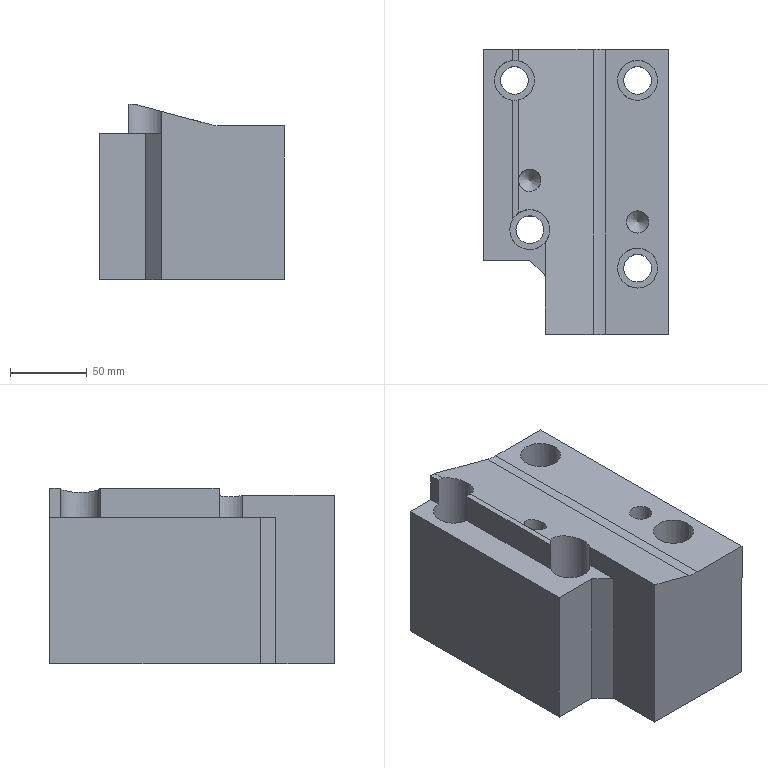Part | STEP file | lll_id5062_x_t | 1 solid | 41 faces | box 120 x 185 x 114 mm | volume 1880331 mm3 | plane 22 | cylinder 15 | cone 2 | torus 2 | commonest cylinder face diameters 18.009 x4 26.008 x4 2 x2 14.506 x2 25 x2 60 x1
STEP:
#1=CARTESIAN_POINT('',(1663.,76.687,-5.));
#2=VERTEX_POINT('',#1);
#3=CARTESIAN_POINT('',(1663.,55.,-5.));
#4=VERTEX_POINT('',#3);
#5=CARTESIAN_POINT('',(1663.,111.,-5.));
#6=DIRECTION('',(0.,-1.,0.));
#7=VECTOR('',#6,1.);
#8=LINE('',#5,#7);
#9=EDGE_CURVE('',#2,#4,#8,.T.);
#10=ORIENTED_EDGE('',*,*,#9,.T.);
#11=CARTESIAN_POINT('',(1663.,55.,-100.));
#12=VERTEX_POINT('',#11);
#13=CARTESIAN_POINT('',(1663.,55.,-80.));
#14=DIRECTION('',(0.,0.,-1.));
#15=VECTOR('',#14,1.);
#16=LINE('',#13,#15);
#17=EDGE_CURVE('',#4,#12,#16,.T.);
#18=ORIENTED_EDGE('',*,*,#17,.T.);
#19=CARTESIAN_POINT('',(1663.,17.,-100.));
#20=VERTEX_POINT('',#19);
#21=CARTESIAN_POINT('',(1663.,111.,-100.));
#22=DIRECTION('',(0.,-1.,0.));
#23=VECTOR('',#22,1.);
#24=LINE('',#21,#23);
#25=EDGE_CURVE('',#12,#20,#24,.T.);
#26=ORIENTED_EDGE('',*,*,#25,.T.);
#27=CARTESIAN_POINT('',(1663.,17.,9.362));
#28=VERTEX_POINT('',#27);
#29=CARTESIAN_POINT('',(1663.,17.,-42.5));
#30=DIRECTION('',(0.,0.,1.));
#31=VECTOR('',#30,1.);
#32=LINE('',#29,#31);
#33=EDGE_CURVE('',#20,#28,#32,.T.);
#34=ORIENTED_EDGE('',*,*,#33,.T.);
#35=CARTESIAN_POINT('',(1663.,76.687,9.362));
#36=VERTEX_POINT('',#35);
#37=CARTESIAN_POINT('',(1663.,22.5,9.362));
#38=DIRECTION('',(0.,1.,0.));
#39=VECTOR('',#38,1.);
#40=LINE('',#37,#39);
#41=EDGE_CURVE('',#28,#36,#40,.T.);
#42=ORIENTED_EDGE('',*,*,#41,.T.);
#43=CARTESIAN_POINT('',(1663.,76.687,3.53));
#44=DIRECTION('',(0.,0.,1.));
#45=VECTOR('',#44,1.);
#46=LINE('',#43,#45);
#47=EDGE_CURVE('',#2,#36,#46,.T.);
#48=ORIENTED_EDGE('',*,*,#47,.F.);
#49=EDGE_LOOP('',(#10,#18,#26,#34,#42,#48));
#50=FACE_OUTER_BOUND('',#49,.T.);
#51=CARTESIAN_POINT('',(1663.,111.,-42.5));
#52=DIRECTION('',(-1.,0.,0.));
#53=DIRECTION('',(0.,0.,-1.));
#54=AXIS2_PLACEMENT_3D('',#51,#52,#53);
#55=PLANE('',#54);
#56=ADVANCED_FACE('',(#50),#55,.T.);
#57=CARTESIAN_POINT('',(1645.691,202.,14.));
#58=VERTEX_POINT('',#57);
#59=CARTESIAN_POINT('',(1642.,202.,14.));
#60=VERTEX_POINT('',#59);
#61=CARTESIAN_POINT('',(1674.,202.,14.));
#62=DIRECTION('',(-1.,0.,0.));
#63=VECTOR('',#62,1.);
#64=LINE('',#61,#63);
#65=EDGE_CURVE('',#58,#60,#64,.T.);
#66=ORIENTED_EDGE('',*,*,#65,.F.);
#67=CARTESIAN_POINT('',(1694.125,202.,1.022));
#68=VERTEX_POINT('',#67);
#69=CARTESIAN_POINT('',(1773.773,202.,-20.319));
#70=DIRECTION('',(0.9659,0.,-0.2588));
#71=VECTOR('',#70,1.);
#72=LINE('',#69,#71);
#73=EDGE_CURVE('',#58,#68,#72,.T.);
#74=ORIENTED_EDGE('',*,*,#73,.T.);
#75=CARTESIAN_POINT('',(1701.89,202.,0.));
#76=VERTEX_POINT('',#75);
#77=CARTESIAN_POINT('',(1701.89,202.,30.));
#78=DIRECTION('',(0.,1.,0.));
#79=DIRECTION('',(0.,0.,1.));
#80=AXIS2_PLACEMENT_3D('',#77,#78,#79);
#81=CIRCLE('',#80,30.);
#82=EDGE_CURVE('',#76,#68,#81,.T.);
#83=ORIENTED_EDGE('',*,*,#82,.F.);
#84=CARTESIAN_POINT('',(1743.,202.,0.));
#85=VERTEX_POINT('',#84);
#86=CARTESIAN_POINT('',(12283.883,202.,0.));
#87=DIRECTION('',(1.,0.,0.));
#88=VECTOR('',#87,1.);
#89=LINE('',#86,#88);
#90=EDGE_CURVE('',#76,#85,#89,.T.);
#91=ORIENTED_EDGE('',*,*,#90,.T.);
#92=CARTESIAN_POINT('',(1743.,202.,-100.));
#93=VERTEX_POINT('',#92);
#94=CARTESIAN_POINT('',(1743.,202.,-32.057));
#95=DIRECTION('',(0.,0.,-1.));
#96=VECTOR('',#95,1.);
#97=LINE('',#94,#96);
#98=EDGE_CURVE('',#85,#93,#97,.T.);
#99=ORIENTED_EDGE('',*,*,#98,.T.);
#100=CARTESIAN_POINT('',(1623.,202.,-100.));
#101=VERTEX_POINT('',#100);
#102=CARTESIAN_POINT('',(1674.,202.,-100.));
#103=DIRECTION('',(-1.,0.,0.));
#104=VECTOR('',#103,1.);
#105=LINE('',#102,#104);
#106=EDGE_CURVE('',#93,#101,#105,.T.);
#107=ORIENTED_EDGE('',*,*,#106,.T.);
#108=CARTESIAN_POINT('',(1623.,202.,-5.));
#109=VERTEX_POINT('',#108);
#110=CARTESIAN_POINT('',(1623.,202.,-80.));
#111=DIRECTION('',(0.,0.,-1.));
#112=VECTOR('',#111,1.);
#113=LINE('',#110,#112);
#114=EDGE_CURVE('',#109,#101,#113,.T.);
#115=ORIENTED_EDGE('',*,*,#114,.F.);
#116=CARTESIAN_POINT('',(1642.,202.,-5.));
#117=VERTEX_POINT('',#116);
#118=CARTESIAN_POINT('',(1674.,202.,-5.));
#119=DIRECTION('',(1.,0.,0.));
#120=VECTOR('',#119,1.);
#121=LINE('',#118,#120);
#122=EDGE_CURVE('',#109,#117,#121,.T.);
#123=ORIENTED_EDGE('',*,*,#122,.T.);
#124=CARTESIAN_POINT('',(1642.,202.,-33.25));
#125=DIRECTION('',(0.,0.,-1.));
#126=VECTOR('',#125,1.);
#127=LINE('',#124,#126);
#128=EDGE_CURVE('',#60,#117,#127,.T.);
#129=ORIENTED_EDGE('',*,*,#128,.F.);
#130=EDGE_LOOP('',(#66,#74,#83,#91,#99,#107,#115,#123,#129));
#131=FACE_OUTER_BOUND('',#130,.T.);
#132=CARTESIAN_POINT('',(1674.,202.,-34.988));
#133=DIRECTION('',(0.,1.,0.));
#134=DIRECTION('',(0.,0.,-1.));
#135=AXIS2_PLACEMENT_3D('',#132,#133,#134);
#136=PLANE('',#135);
#137=ADVANCED_FACE('',(#131),#136,.T.);
#138=CARTESIAN_POINT('',(1694.125,17.,1.022));
#139=VERTEX_POINT('',#138);
#140=CARTESIAN_POINT('',(1773.773,17.,-20.319));
#141=DIRECTION('',(-0.9659,0.,0.2588));
#142=VECTOR('',#141,1.);
#143=LINE('',#140,#142);
#144=EDGE_CURVE('',#139,#28,#143,.T.);
#145=ORIENTED_EDGE('',*,*,#144,.T.);
#146=ORIENTED_EDGE('',*,*,#33,.F.);
#147=CARTESIAN_POINT('',(1743.,17.,-100.));
#148=VERTEX_POINT('',#147);
#149=CARTESIAN_POINT('',(1644.,17.,-100.));
#150=DIRECTION('',(1.,0.,0.));
#151=VECTOR('',#150,1.);
#152=LINE('',#149,#151);
#153=EDGE_CURVE('',#20,#148,#152,.T.);
#154=ORIENTED_EDGE('',*,*,#153,.T.);
#155=CARTESIAN_POINT('',(1743.,17.,0.));
#156=VERTEX_POINT('',#155);
#157=CARTESIAN_POINT('',(1743.,17.,-80.));
#158=DIRECTION('',(0.,0.,-1.));
#159=VECTOR('',#158,1.);
#160=LINE('',#157,#159);
#161=EDGE_CURVE('',#156,#148,#160,.T.);
#162=ORIENTED_EDGE('',*,*,#161,.F.);
#163=CARTESIAN_POINT('',(1701.89,17.,0.));
#164=VERTEX_POINT('',#163);
#165=CARTESIAN_POINT('',(12283.883,17.,0.));
#166=DIRECTION('',(-1.,0.,0.));
#167=VECTOR('',#166,1.);
#168=LINE('',#165,#167);
#169=EDGE_CURVE('',#156,#164,#168,.T.);
#170=ORIENTED_EDGE('',*,*,#169,.T.);
#171=CARTESIAN_POINT('',(1701.89,17.,30.));
#172=DIRECTION('',(0.,1.,0.));
#173=DIRECTION('',(0.,0.,-1.));
#174=AXIS2_PLACEMENT_3D('',#171,#172,#173);
#175=CIRCLE('',#174,30.);
#176=EDGE_CURVE('',#164,#139,#175,.T.);
#177=ORIENTED_EDGE('',*,*,#176,.T.);
#178=EDGE_LOOP('',(#145,#146,#154,#162,#170,#177));
#179=FACE_OUTER_BOUND('',#178,.T.);
#180=CARTESIAN_POINT('',(1644.,17.,-80.));
#181=DIRECTION('',(0.,-1.,0.));
#182=DIRECTION('',(0.,0.,1.));
#183=AXIS2_PLACEMENT_3D('',#180,#181,#182);
#184=PLANE('',#183);
#185=ADVANCED_FACE('',(#179),#184,.T.);
#186=ORIENTED_EDGE('',*,*,#73,.F.);
#187=CARTESIAN_POINT('',(1645.691,194.722,14.));
#188=VERTEX_POINT('',#187);
#189=CARTESIAN_POINT('',(1645.691,22.5,14.));
#190=DIRECTION('',(0.,-1.,0.));
#191=VECTOR('',#190,1.);
#192=LINE('',#189,#191);
#193=EDGE_CURVE('',#58,#188,#192,.T.);
#194=ORIENTED_EDGE('',*,*,#193,.T.);
#195=CARTESIAN_POINT('',(1645.691,169.277,14.));
#196=VERTEX_POINT('',#195);
#197=CARTESIAN_POINT('',(1643.,182.,14.721));
#198=DIRECTION('',(-0.2588,0.,-0.9659));
#199=DIRECTION('',(0.9659,0.,-0.2588));
#200=AXIS2_PLACEMENT_3D('',#197,#198,#199);
#201=ELLIPSE('',#200,13.463,13.004);
#202=EDGE_CURVE('',#188,#196,#201,.T.);
#203=ORIENTED_EDGE('',*,*,#202,.T.);
#204=CARTESIAN_POINT('',(1645.691,95.756,14.));
#205=VERTEX_POINT('',#204);
#206=CARTESIAN_POINT('',(1645.691,22.5,14.));
#207=DIRECTION('',(0.,-1.,0.));
#208=VECTOR('',#207,1.);
#209=LINE('',#206,#208);
#210=EDGE_CURVE('',#196,#205,#209,.T.);
#211=ORIENTED_EDGE('',*,*,#210,.T.);
#212=CARTESIAN_POINT('',(1653.,85.,12.042));
#213=DIRECTION('',(-0.2588,0.,-0.9659));
#214=DIRECTION('',(0.9659,0.,-0.2588));
#215=AXIS2_PLACEMENT_3D('',#212,#213,#214);
#216=ELLIPSE('',#215,13.463,13.004);
#217=EDGE_CURVE('',#205,#36,#216,.T.);
#218=ORIENTED_EDGE('',*,*,#217,.T.);
#219=ORIENTED_EDGE('',*,*,#41,.F.);
#220=ORIENTED_EDGE('',*,*,#144,.F.);
#221=CARTESIAN_POINT('',(1694.125,22.5,1.022));
#222=DIRECTION('',(0.,-1.,0.));
#223=VECTOR('',#222,1.);
#224=LINE('',#221,#223);
#225=EDGE_CURVE('',#68,#139,#224,.T.);
#226=ORIENTED_EDGE('',*,*,#225,.F.);
#227=EDGE_LOOP('',(#186,#194,#203,#211,#218,#219,#220,#226));
#228=FACE_BOUND('',#227,.T.);
#229=CARTESIAN_POINT('',(1660.253,117.,10.098));
#230=VERTEX_POINT('',#229);
#231=CARTESIAN_POINT('',(1653.,117.,12.042));
#232=DIRECTION('',(-0.2588,0.,-0.9659));
#233=DIRECTION('',(0.9659,0.,-0.2588));
#234=AXIS2_PLACEMENT_3D('',#231,#232,#233);
#235=ELLIPSE('',#234,7.509,7.253);
#236=EDGE_CURVE('',#230,#230,#235,.T.);
#237=ORIENTED_EDGE('',*,*,#236,.T.);
#238=EDGE_LOOP('',(#237));
#239=FACE_BOUND('',#238,.T.);
#240=CARTESIAN_POINT('',(1773.773,22.5,-20.319));
#241=DIRECTION('',(-0.2588,0.,-0.9659));
#242=DIRECTION('',(0.9659,0.,-0.2588));
#243=AXIS2_PLACEMENT_3D('',#240,#241,#242);
#244=PLANE('',#243);
#245=ADVANCED_FACE('',(#228,#239),#244,.F.);
#246=CARTESIAN_POINT('',(1660.,122.,-100.));
#247=VERTEX_POINT('',#246);
#248=CARTESIAN_POINT('',(1660.,147.,-100.));
#249=VERTEX_POINT('',#248);
#250=CARTESIAN_POINT('',(1660.,134.5,-100.));
#251=DIRECTION('',(0.,0.,-1.));
#252=DIRECTION('',(-1.,0.,0.));
#253=AXIS2_PLACEMENT_3D('',#250,#251,#252);
#254=CIRCLE('',#253,12.5);
#255=EDGE_CURVE('',#247,#249,#254,.T.);
#256=ORIENTED_EDGE('',*,*,#255,.F.);
#257=CARTESIAN_POINT('',(1716.,122.,-100.));
#258=VERTEX_POINT('',#257);
#259=CARTESIAN_POINT('',(-2196.249,122.,-100.));
#260=DIRECTION('',(-1.,0.,0.));
#261=VECTOR('',#260,1.);
#262=LINE('',#259,#261);
#263=EDGE_CURVE('',#258,#247,#262,.T.);
#264=ORIENTED_EDGE('',*,*,#263,.F.);
#265=CARTESIAN_POINT('',(1716.,147.,-100.));
#266=VERTEX_POINT('',#265);
#267=CARTESIAN_POINT('',(1716.,134.5,-100.));
#268=DIRECTION('',(0.,0.,-1.));
#269=DIRECTION('',(-1.,0.,0.));
#270=AXIS2_PLACEMENT_3D('',#267,#268,#269);
#271=CIRCLE('',#270,12.5);
#272=EDGE_CURVE('',#266,#258,#271,.T.);
#273=ORIENTED_EDGE('',*,*,#272,.F.);
#274=CARTESIAN_POINT('',(-2196.249,147.,-100.));
#275=DIRECTION('',(1.,0.,0.));
#276=VECTOR('',#275,1.);
#277=LINE('',#274,#276);
#278=EDGE_CURVE('',#249,#266,#277,.T.);
#279=ORIENTED_EDGE('',*,*,#278,.F.);
#280=EDGE_LOOP('',(#256,#264,#273,#279));
#281=FACE_BOUND('',#280,.T.);
#282=CARTESIAN_POINT('',(1713.995,182.,-100.));
#283=VERTEX_POINT('',#282);
#284=CARTESIAN_POINT('',(1723.,182.,-100.));
#285=DIRECTION('',(0.,0.,-1.));
#286=DIRECTION('',(-1.,0.,0.));
#287=AXIS2_PLACEMENT_3D('',#284,#285,#286);
#288=CIRCLE('',#287,9.005);
#289=EDGE_CURVE('',#283,#283,#288,.T.);
#290=ORIENTED_EDGE('',*,*,#289,.F.);
#291=EDGE_LOOP('',(#290));
#292=FACE_BOUND('',#291,.T.);
#293=CARTESIAN_POINT('',(1713.995,60.,-100.));
#294=VERTEX_POINT('',#293);
#295=CARTESIAN_POINT('',(1723.,60.,-100.));
#296=DIRECTION('',(0.,0.,-1.));
#297=DIRECTION('',(-1.,0.,0.));
#298=AXIS2_PLACEMENT_3D('',#295,#296,#297);
#299=CIRCLE('',#298,9.005);
#300=EDGE_CURVE('',#294,#294,#299,.T.);
#301=ORIENTED_EDGE('',*,*,#300,.F.);
#302=EDGE_LOOP('',(#301));
#303=FACE_BOUND('',#302,.T.);
#304=ORIENTED_EDGE('',*,*,#153,.F.);
#305=ORIENTED_EDGE('',*,*,#25,.F.);
#306=CARTESIAN_POINT('',(1653.,65.,-100.));
#307=VERTEX_POINT('',#306);
#308=CARTESIAN_POINT('',(1653.,65.,-100.));
#309=DIRECTION('',(-0.7071,0.7071,0.));
#310=VECTOR('',#309,1.);
#311=LINE('',#308,#310);
#312=EDGE_CURVE('',#12,#307,#311,.T.);
#313=ORIENTED_EDGE('',*,*,#312,.T.);
#314=CARTESIAN_POINT('',(1623.,65.,-100.));
#315=VERTEX_POINT('',#314);
#316=CARTESIAN_POINT('',(1644.,65.,-100.));
#317=DIRECTION('',(1.,0.,0.));
#318=VECTOR('',#317,1.);
#319=LINE('',#316,#318);
#320=EDGE_CURVE('',#315,#307,#319,.T.);
#321=ORIENTED_EDGE('',*,*,#320,.F.);
#322=CARTESIAN_POINT('',(1623.,320.,-100.));
#323=DIRECTION('',(0.,-1.,0.));
#324=VECTOR('',#323,1.);
#325=LINE('',#322,#324);
#326=EDGE_CURVE('',#101,#315,#325,.T.);
#327=ORIENTED_EDGE('',*,*,#326,.F.);
#328=ORIENTED_EDGE('',*,*,#106,.F.);
#329=CARTESIAN_POINT('',(1743.,187.,-100.));
#330=DIRECTION('',(0.,-1.,0.));
#331=VECTOR('',#330,1.);
#332=LINE('',#329,#331);
#333=EDGE_CURVE('',#93,#148,#332,.T.);
#334=ORIENTED_EDGE('',*,*,#333,.T.);
#335=EDGE_LOOP('',(#304,#305,#313,#321,#327,#328,#334));
#336=FACE_BOUND('',#335,.T.);
#337=CARTESIAN_POINT('',(1643.995,85.,-100.));
#338=VERTEX_POINT('',#337);
#339=CARTESIAN_POINT('',(1653.,85.,-100.));
#340=DIRECTION('',(0.,0.,-1.));
#341=DIRECTION('',(-1.,0.,0.));
#342=AXIS2_PLACEMENT_3D('',#339,#340,#341);
#343=CIRCLE('',#342,9.005);
#344=EDGE_CURVE('',#338,#338,#343,.T.);
#345=ORIENTED_EDGE('',*,*,#344,.F.);
#346=EDGE_LOOP('',(#345));
#347=FACE_BOUND('',#346,.T.);
#348=CARTESIAN_POINT('',(1633.995,182.,-100.));
#349=VERTEX_POINT('',#348);
#350=CARTESIAN_POINT('',(1643.,182.,-100.));
#351=DIRECTION('',(0.,0.,-1.));
#352=DIRECTION('',(-1.,0.,0.));
#353=AXIS2_PLACEMENT_3D('',#350,#351,#352);
#354=CIRCLE('',#353,9.005);
#355=EDGE_CURVE('',#349,#349,#354,.T.);
#356=ORIENTED_EDGE('',*,*,#355,.F.);
#357=EDGE_LOOP('',(#356));
#358=FACE_BOUND('',#357,.T.);
#359=CARTESIAN_POINT('',(-2196.249,1.,-100.));
#360=DIRECTION('',(0.,0.,-1.));
#361=DIRECTION('',(1.,0.,0.));
#362=AXIS2_PLACEMENT_3D('',#359,#360,#361);
#363=PLANE('',#362);
#364=ADVANCED_FACE('',(#281,#292,#303,#336,#347,#358),#363,.T.);
#365=ORIENTED_EDGE('',*,*,#217,.F.);
#366=CARTESIAN_POINT('',(1642.,91.936,14.));
#367=VERTEX_POINT('',#366);
#368=CARTESIAN_POINT('',(1653.,85.,14.));
#369=DIRECTION('',(0.,0.,-1.));
#370=DIRECTION('',(-1.,0.,0.));
#371=AXIS2_PLACEMENT_3D('',#368,#369,#370);
#372=CIRCLE('',#371,13.004);
#373=EDGE_CURVE('',#367,#205,#372,.T.);
#374=ORIENTED_EDGE('',*,*,#373,.F.);
#375=CARTESIAN_POINT('',(1642.,91.936,-5.));
#376=VERTEX_POINT('',#375);
#377=CARTESIAN_POINT('',(1642.,91.936,13.5));
#378=DIRECTION('',(0.,0.,-1.));
#379=VECTOR('',#378,1.);
#380=LINE('',#377,#379);
#381=EDGE_CURVE('',#367,#376,#380,.T.);
#382=ORIENTED_EDGE('',*,*,#381,.T.);
#383=CARTESIAN_POINT('',(1653.,85.,-5.));
#384=DIRECTION('',(0.,0.,1.));
#385=DIRECTION('',(1.,0.,0.));
#386=AXIS2_PLACEMENT_3D('',#383,#384,#385);
#387=CIRCLE('',#386,13.004);
#388=EDGE_CURVE('',#376,#2,#387,.T.);
#389=ORIENTED_EDGE('',*,*,#388,.T.);
#390=ORIENTED_EDGE('',*,*,#47,.T.);
#391=EDGE_LOOP('',(#365,#374,#382,#389,#390));
#392=FACE_BOUND('',#391,.T.);
#393=CARTESIAN_POINT('',(1639.996,85.,-50.));
#394=VERTEX_POINT('',#393);
#395=CARTESIAN_POINT('',(1653.,85.,-50.));
#396=DIRECTION('',(0.,0.,-1.));
#397=DIRECTION('',(-1.,0.,0.));
#398=AXIS2_PLACEMENT_3D('',#395,#396,#397);
#399=CIRCLE('',#398,13.004);
#400=EDGE_CURVE('',#394,#394,#399,.T.);
#401=ORIENTED_EDGE('',*,*,#400,.T.);
#402=EDGE_LOOP('',(#401));
#403=FACE_BOUND('',#402,.T.);
#404=CARTESIAN_POINT('',(1653.,85.,13.5));
#405=DIRECTION('',(0.,0.,-1.));
#406=DIRECTION('',(-1.,0.,0.));
#407=AXIS2_PLACEMENT_3D('',#404,#405,#406);
#408=CYLINDRICAL_SURFACE('',#407,13.004);
#409=ADVANCED_FACE('',(#392,#403),#408,.F.);
#410=ORIENTED_EDGE('',*,*,#400,.F.);
#411=EDGE_LOOP('',(#410));
#412=FACE_BOUND('',#411,.T.);
#413=CARTESIAN_POINT('',(1662.005,85.,-50.));
#414=VERTEX_POINT('',#413);
#415=CARTESIAN_POINT('',(1653.,85.,-50.));
#416=DIRECTION('',(0.,0.,-1.));
#417=DIRECTION('',(1.,0.,0.));
#418=AXIS2_PLACEMENT_3D('',#415,#416,#417);
#419=CIRCLE('',#418,9.005);
#420=EDGE_CURVE('',#414,#414,#419,.T.);
#421=ORIENTED_EDGE('',*,*,#420,.T.);
#422=EDGE_LOOP('',(#421));
#423=FACE_BOUND('',#422,.T.);
#424=CARTESIAN_POINT('',(1653.,85.,-50.));
#425=DIRECTION('',(0.,0.,-1.));
#426=DIRECTION('',(1.,0.,0.));
#427=AXIS2_PLACEMENT_3D('',#424,#425,#426);
#428=PLANE('',#427);
#429=ADVANCED_FACE('',(#412,#423),#428,.F.);
#430=ORIENTED_EDGE('',*,*,#98,.F.);
#431=CARTESIAN_POINT('',(1743.,-13712.786,0.));
#432=DIRECTION('',(0.,1.,0.));
#433=VECTOR('',#432,1.);
#434=LINE('',#431,#433);
#435=EDGE_CURVE('',#156,#85,#434,.T.);
#436=ORIENTED_EDGE('',*,*,#435,.F.);
#437=ORIENTED_EDGE('',*,*,#161,.T.);
#438=ORIENTED_EDGE('',*,*,#333,.F.);
#439=EDGE_LOOP('',(#430,#436,#437,#438));
#440=FACE_OUTER_BOUND('',#439,.T.);
#441=CARTESIAN_POINT('',(1743.,187.,-32.057));
#442=DIRECTION('',(-1.,0.,0.));
#443=DIRECTION('',(0.,0.,-1.));
#444=AXIS2_PLACEMENT_3D('',#441,#442,#443);
#445=PLANE('',#444);
#446=ADVANCED_FACE('',(#440),#445,.F.);
#447=CARTESIAN_POINT('',(1723.,82.747,0.));
#448=VERTEX_POINT('',#447);
#449=CARTESIAN_POINT('',(1723.,90.,0.));
#450=DIRECTION('',(0.,0.,-1.));
#451=DIRECTION('',(0.,-1.,0.));
#452=AXIS2_PLACEMENT_3D('',#449,#450,#451);
#453=CIRCLE('',#452,7.253);
#454=EDGE_CURVE('',#448,#448,#453,.T.);
#455=ORIENTED_EDGE('',*,*,#454,.T.);
#456=EDGE_LOOP('',(#455));
#457=FACE_BOUND('',#456,.T.);
#458=CARTESIAN_POINT('',(1723.,168.996,0.));
#459=VERTEX_POINT('',#458);
#460=CARTESIAN_POINT('',(1723.,182.,0.));
#461=DIRECTION('',(0.,0.,-1.));
#462=DIRECTION('',(0.,-1.,0.));
#463=AXIS2_PLACEMENT_3D('',#460,#461,#462);
#464=CIRCLE('',#463,13.004);
#465=EDGE_CURVE('',#459,#459,#464,.T.);
#466=ORIENTED_EDGE('',*,*,#465,.T.);
#467=EDGE_LOOP('',(#466));
#468=FACE_BOUND('',#467,.T.);
#469=CARTESIAN_POINT('',(1723.,46.996,0.));
#470=VERTEX_POINT('',#469);
#471=CARTESIAN_POINT('',(1723.,60.,0.));
#472=DIRECTION('',(0.,0.,-1.));
#473=DIRECTION('',(0.,-1.,0.));
#474=AXIS2_PLACEMENT_3D('',#471,#472,#473);
#475=CIRCLE('',#474,13.004);
#476=EDGE_CURVE('',#470,#470,#475,.T.);
#477=ORIENTED_EDGE('',*,*,#476,.T.);
#478=EDGE_LOOP('',(#477));
#479=FACE_BOUND('',#478,.T.);
#480=ORIENTED_EDGE('',*,*,#90,.F.);
#481=CARTESIAN_POINT('',(1701.89,22.5,0.));
#482=DIRECTION('',(0.,-1.,0.));
#483=VECTOR('',#482,1.);
#484=LINE('',#481,#483);
#485=EDGE_CURVE('',#76,#164,#484,.T.);
#486=ORIENTED_EDGE('',*,*,#485,.T.);
#487=ORIENTED_EDGE('',*,*,#169,.F.);
#488=ORIENTED_EDGE('',*,*,#435,.T.);
#489=EDGE_LOOP('',(#480,#486,#487,#488));
#490=FACE_BOUND('',#489,.T.);
#491=CARTESIAN_POINT('',(12283.883,-13712.786,0.));
#492=DIRECTION('',(0.,0.,-1.));
#493=DIRECTION('',(1.,0.,0.));
#494=AXIS2_PLACEMENT_3D('',#491,#492,#493);
#495=PLANE('',#494);
#496=ADVANCED_FACE('',(#457,#468,#479,#490),#495,.F.);
#497=ORIENTED_EDGE('',*,*,#82,.T.);
#498=ORIENTED_EDGE('',*,*,#225,.T.);
#499=ORIENTED_EDGE('',*,*,#176,.F.);
#500=ORIENTED_EDGE('',*,*,#485,.F.);
#501=EDGE_LOOP('',(#497,#498,#499,#500));
#502=FACE_OUTER_BOUND('',#501,.T.);
#503=CARTESIAN_POINT('',(1701.89,22.5,30.));
#504=DIRECTION('',(0.,-1.,0.));
#505=DIRECTION('',(-1.,0.,0.));
#506=AXIS2_PLACEMENT_3D('',#503,#504,#505);
#507=CYLINDRICAL_SURFACE('',#506,30.);
#508=ADVANCED_FACE('',(#502),#507,.F.);
#509=CARTESIAN_POINT('',(1709.996,60.,-50.));
#510=VERTEX_POINT('',#509);
#511=CARTESIAN_POINT('',(1723.,60.,-50.));
#512=DIRECTION('',(0.,0.,-1.));
#513=DIRECTION('',(-1.,0.,0.));
#514=AXIS2_PLACEMENT_3D('',#511,#512,#513);
#515=CIRCLE('',#514,13.004);
#516=EDGE_CURVE('',#510,#510,#515,.T.);
#517=ORIENTED_EDGE('',*,*,#516,.T.);
#518=EDGE_LOOP('',(#517));
#519=FACE_BOUND('',#518,.T.);
#520=ORIENTED_EDGE('',*,*,#476,.F.);
#521=EDGE_LOOP('',(#520));
#522=FACE_BOUND('',#521,.T.);
#523=CARTESIAN_POINT('',(1723.,60.,13.5));
#524=DIRECTION('',(0.,0.,-1.));
#525=DIRECTION('',(-1.,0.,0.));
#526=AXIS2_PLACEMENT_3D('',#523,#524,#525);
#527=CYLINDRICAL_SURFACE('',#526,13.004);
#528=ADVANCED_FACE('',(#519,#522),#527,.F.);
#529=ORIENTED_EDGE('',*,*,#300,.T.);
#530=EDGE_LOOP('',(#529));
#531=FACE_BOUND('',#530,.T.);
#532=CARTESIAN_POINT('',(1732.005,60.,-50.));
#533=VERTEX_POINT('',#532);
#534=CARTESIAN_POINT('',(1723.,60.,-50.));
#535=DIRECTION('',(0.,0.,-1.));
#536=DIRECTION('',(1.,0.,0.));
#537=AXIS2_PLACEMENT_3D('',#534,#535,#536);
#538=CIRCLE('',#537,9.005);
#539=EDGE_CURVE('',#533,#533,#538,.T.);
#540=ORIENTED_EDGE('',*,*,#539,.F.);
#541=EDGE_LOOP('',(#540));
#542=FACE_BOUND('',#541,.T.);
#543=CARTESIAN_POINT('',(1723.,60.,15.5));
#544=DIRECTION('',(0.,0.,-1.));
#545=DIRECTION('',(-1.,0.,0.));
#546=AXIS2_PLACEMENT_3D('',#543,#544,#545);
#547=CYLINDRICAL_SURFACE('',#546,9.005);
#548=ADVANCED_FACE('',(#531,#542),#547,.F.);
#549=ORIENTED_EDGE('',*,*,#539,.T.);
#550=EDGE_LOOP('',(#549));
#551=FACE_BOUND('',#550,.T.);
#552=ORIENTED_EDGE('',*,*,#516,.F.);
#553=EDGE_LOOP('',(#552));
#554=FACE_BOUND('',#553,.T.);
#555=CARTESIAN_POINT('',(1723.,40.,-50.));
#556=DIRECTION('',(0.,0.,-1.));
#557=DIRECTION('',(1.,0.,0.));
#558=AXIS2_PLACEMENT_3D('',#555,#556,#557);
#559=PLANE('',#558);
#560=ADVANCED_FACE('',(#551,#554),#559,.F.);
#561=CARTESIAN_POINT('',(1736.004,182.,-50.));
#562=VERTEX_POINT('',#561);
#563=CARTESIAN_POINT('',(1723.,182.,-50.));
#564=DIRECTION('',(0.,0.,-1.));
#565=DIRECTION('',(1.,0.,0.));
#566=AXIS2_PLACEMENT_3D('',#563,#564,#565);
#567=CIRCLE('',#566,13.004);
#568=EDGE_CURVE('',#562,#562,#567,.T.);
#569=ORIENTED_EDGE('',*,*,#568,.T.);
#570=EDGE_LOOP('',(#569));
#571=FACE_BOUND('',#570,.T.);
#572=ORIENTED_EDGE('',*,*,#465,.F.);
#573=EDGE_LOOP('',(#572));
#574=FACE_BOUND('',#573,.T.);
#575=CARTESIAN_POINT('',(1723.,182.,13.5));
#576=DIRECTION('',(0.,0.,-1.));
#577=DIRECTION('',(-1.,0.,0.));
#578=AXIS2_PLACEMENT_3D('',#575,#576,#577);
#579=CYLINDRICAL_SURFACE('',#578,13.004);
#580=ADVANCED_FACE('',(#571,#574),#579,.F.);
#581=ORIENTED_EDGE('',*,*,#289,.T.);
#582=EDGE_LOOP('',(#581));
#583=FACE_BOUND('',#582,.T.);
#584=CARTESIAN_POINT('',(1732.005,182.,-50.));
#585=VERTEX_POINT('',#584);
#586=CARTESIAN_POINT('',(1723.,182.,-50.));
#587=DIRECTION('',(0.,0.,-1.));
#588=DIRECTION('',(1.,0.,0.));
#589=AXIS2_PLACEMENT_3D('',#586,#587,#588);
#590=CIRCLE('',#589,9.005);
#591=EDGE_CURVE('',#585,#585,#590,.T.);
#592=ORIENTED_EDGE('',*,*,#591,.F.);
#593=EDGE_LOOP('',(#592));
#594=FACE_BOUND('',#593,.T.);
#595=CARTESIAN_POINT('',(1723.,182.,15.5));
#596=DIRECTION('',(0.,0.,-1.));
#597=DIRECTION('',(-1.,0.,0.));
#598=AXIS2_PLACEMENT_3D('',#595,#596,#597);
#599=CYLINDRICAL_SURFACE('',#598,9.005);
#600=ADVANCED_FACE('',(#583,#594),#599,.F.);
#601=ORIENTED_EDGE('',*,*,#591,.T.);
#602=EDGE_LOOP('',(#601));
#603=FACE_BOUND('',#602,.T.);
#604=ORIENTED_EDGE('',*,*,#568,.F.);
#605=EDGE_LOOP('',(#604));
#606=FACE_BOUND('',#605,.T.);
#607=CARTESIAN_POINT('',(1723.,182.,-50.));
#608=DIRECTION('',(0.,0.,-1.));
#609=DIRECTION('',(1.,0.,0.));
#610=AXIS2_PLACEMENT_3D('',#607,#608,#609);
#611=PLANE('',#610);
#612=ADVANCED_FACE('',(#603,#606),#611,.F.);
#613=CARTESIAN_POINT('',(1730.253,90.,-22.253));
#614=VERTEX_POINT('',#613);
#615=CARTESIAN_POINT('',(1723.,90.,-22.253));
#616=DIRECTION('',(0.,0.,-1.));
#617=DIRECTION('',(1.,0.,0.));
#618=AXIS2_PLACEMENT_3D('',#615,#616,#617);
#619=CIRCLE('',#618,7.253);
#620=EDGE_CURVE('',#614,#614,#619,.T.);
#621=ORIENTED_EDGE('',*,*,#620,.T.);
#622=EDGE_LOOP('',(#621));
#623=FACE_BOUND('',#622,.T.);
#624=ORIENTED_EDGE('',*,*,#454,.F.);
#625=EDGE_LOOP('',(#624));
#626=FACE_BOUND('',#625,.T.);
#627=CARTESIAN_POINT('',(1723.,90.,15.5));
#628=DIRECTION('',(0.,0.,-1.));
#629=DIRECTION('',(-1.,0.,0.));
#630=AXIS2_PLACEMENT_3D('',#627,#628,#629);
#631=CYLINDRICAL_SURFACE('',#630,7.253);
#632=ADVANCED_FACE('',(#623,#626),#631,.F.);
#633=CARTESIAN_POINT('',(1723.,90.,-29.506));
#634=VERTEX_POINT('',#633);
#635=VERTEX_LOOP('',#634);
#636=FACE_BOUND('',#635,.T.);
#637=ORIENTED_EDGE('',*,*,#620,.F.);
#638=EDGE_LOOP('',(#637));
#639=FACE_BOUND('',#638,.T.);
#640=CARTESIAN_POINT('',(1723.,90.,-22.253));
#641=DIRECTION('',(0.,0.,1.));
#642=DIRECTION('',(-1.,0.,0.));
#643=AXIS2_PLACEMENT_3D('',#640,#641,#642);
#644=CONICAL_SURFACE('',#643,7.253,45.);
#645=ADVANCED_FACE('',(#636,#639),#644,.F.);
#646=CARTESIAN_POINT('',(1653.,117.,-29.506));
#647=VERTEX_POINT('',#646);
#648=VERTEX_LOOP('',#647);
#649=FACE_BOUND('',#648,.T.);
#650=CARTESIAN_POINT('',(1660.253,117.,-22.253));
#651=VERTEX_POINT('',#650);
#652=CARTESIAN_POINT('',(1653.,117.,-22.253));
#653=DIRECTION('',(0.,0.,1.));
#654=DIRECTION('',(1.,0.,0.));
#655=AXIS2_PLACEMENT_3D('',#652,#653,#654);
#656=CIRCLE('',#655,7.253);
#657=EDGE_CURVE('',#651,#651,#656,.T.);
#658=ORIENTED_EDGE('',*,*,#657,.T.);
#659=EDGE_LOOP('',(#658));
#660=FACE_BOUND('',#659,.T.);
#661=CARTESIAN_POINT('',(1653.,117.,-22.253));
#662=DIRECTION('',(0.,0.,1.));
#663=DIRECTION('',(-1.,0.,0.));
#664=AXIS2_PLACEMENT_3D('',#661,#662,#663);
#665=CONICAL_SURFACE('',#664,7.253,45.);
#666=ADVANCED_FACE('',(#649,#660),#665,.F.);
#667=CARTESIAN_POINT('',(1629.996,182.,-50.));
#668=VERTEX_POINT('',#667);
#669=CARTESIAN_POINT('',(1643.,182.,-50.));
#670=DIRECTION('',(0.,0.,-1.));
#671=DIRECTION('',(-1.,0.,0.));
#672=AXIS2_PLACEMENT_3D('',#669,#670,#671);
#673=CIRCLE('',#672,13.004);
#674=EDGE_CURVE('',#668,#668,#673,.T.);
#675=ORIENTED_EDGE('',*,*,#674,.F.);
#676=EDGE_LOOP('',(#675));
#677=FACE_BOUND('',#676,.T.);
#678=CARTESIAN_POINT('',(1652.005,182.,-50.));
#679=VERTEX_POINT('',#678);
#680=CARTESIAN_POINT('',(1643.,182.,-50.));
#681=DIRECTION('',(0.,0.,-1.));
#682=DIRECTION('',(1.,0.,0.));
#683=AXIS2_PLACEMENT_3D('',#680,#681,#682);
#684=CIRCLE('',#683,9.005);
#685=EDGE_CURVE('',#679,#679,#684,.T.);
#686=ORIENTED_EDGE('',*,*,#685,.T.);
#687=EDGE_LOOP('',(#686));
#688=FACE_BOUND('',#687,.T.);
#689=CARTESIAN_POINT('',(1643.,182.,-50.));
#690=DIRECTION('',(0.,0.,-1.));
#691=DIRECTION('',(1.,0.,0.));
#692=AXIS2_PLACEMENT_3D('',#689,#690,#691);
#693=PLANE('',#692);
#694=ADVANCED_FACE('',(#677,#688),#693,.F.);
#695=CARTESIAN_POINT('',(1642.,169.034,14.));
#696=VERTEX_POINT('',#695);
#697=CARTESIAN_POINT('',(1642.,169.034,-5.));
#698=VERTEX_POINT('',#697);
#699=CARTESIAN_POINT('',(1642.,169.034,13.5));
#700=DIRECTION('',(0.,0.,-1.));
#701=VECTOR('',#700,1.);
#702=LINE('',#699,#701);
#703=EDGE_CURVE('',#696,#698,#702,.T.);
#704=ORIENTED_EDGE('',*,*,#703,.F.);
#705=CARTESIAN_POINT('',(1643.,182.,14.));
#706=DIRECTION('',(0.,0.,1.));
#707=DIRECTION('',(-1.,0.,0.));
#708=AXIS2_PLACEMENT_3D('',#705,#706,#707);
#709=CIRCLE('',#708,13.004);
#710=EDGE_CURVE('',#696,#196,#709,.T.);
#711=ORIENTED_EDGE('',*,*,#710,.T.);
#712=ORIENTED_EDGE('',*,*,#202,.F.);
#713=CARTESIAN_POINT('',(1642.,194.965,14.));
#714=VERTEX_POINT('',#713);
#715=CARTESIAN_POINT('',(1643.,182.,14.));
#716=DIRECTION('',(0.,0.,1.));
#717=DIRECTION('',(-1.,0.,0.));
#718=AXIS2_PLACEMENT_3D('',#715,#716,#717);
#719=CIRCLE('',#718,13.004);
#720=EDGE_CURVE('',#188,#714,#719,.T.);
#721=ORIENTED_EDGE('',*,*,#720,.T.);
#722=CARTESIAN_POINT('',(1642.,194.965,-5.));
#723=VERTEX_POINT('',#722);
#724=CARTESIAN_POINT('',(1642.,194.965,13.5));
#725=DIRECTION('',(0.,0.,1.));
#726=VECTOR('',#725,1.);
#727=LINE('',#724,#726);
#728=EDGE_CURVE('',#723,#714,#727,.T.);
#729=ORIENTED_EDGE('',*,*,#728,.F.);
#730=CARTESIAN_POINT('',(1643.,182.,-5.));
#731=DIRECTION('',(0.,0.,-1.));
#732=DIRECTION('',(1.,0.,0.));
#733=AXIS2_PLACEMENT_3D('',#730,#731,#732);
#734=CIRCLE('',#733,13.004);
#735=EDGE_CURVE('',#698,#723,#734,.T.);
#736=ORIENTED_EDGE('',*,*,#735,.F.);
#737=EDGE_LOOP('',(#704,#711,#712,#721,#729,#736));
#738=FACE_BOUND('',#737,.T.);
#739=ORIENTED_EDGE('',*,*,#674,.T.);
#740=EDGE_LOOP('',(#739));
#741=FACE_BOUND('',#740,.T.);
#742=CARTESIAN_POINT('',(1643.,182.,13.5));
#743=DIRECTION('',(0.,0.,-1.));
#744=DIRECTION('',(-1.,0.,0.));
#745=AXIS2_PLACEMENT_3D('',#742,#743,#744);
#746=CYLINDRICAL_SURFACE('',#745,13.004);
#747=ADVANCED_FACE('',(#738,#741),#746,.F.);
#748=CARTESIAN_POINT('',(1642.,111.,14.));
#749=DIRECTION('',(0.,1.,0.));
#750=VECTOR('',#749,1.);
#751=LINE('',#748,#750);
#752=EDGE_CURVE('',#714,#60,#751,.T.);
#753=ORIENTED_EDGE('',*,*,#752,.T.);
#754=ORIENTED_EDGE('',*,*,#128,.T.);
#755=CARTESIAN_POINT('',(1642.,111.,-5.));
#756=DIRECTION('',(0.,-1.,0.));
#757=VECTOR('',#756,1.);
#758=LINE('',#755,#757);
#759=EDGE_CURVE('',#117,#723,#758,.T.);
#760=ORIENTED_EDGE('',*,*,#759,.T.);
#761=ORIENTED_EDGE('',*,*,#728,.T.);
#762=EDGE_LOOP('',(#753,#754,#760,#761));
#763=FACE_OUTER_BOUND('',#762,.T.);
#764=CARTESIAN_POINT('',(1642.,111.,-33.25));
#765=DIRECTION('',(-1.,0.,0.));
#766=DIRECTION('',(0.,0.,-1.));
#767=AXIS2_PLACEMENT_3D('',#764,#765,#766);
#768=PLANE('',#767);
#769=ADVANCED_FACE('',(#763),#768,.T.);
#770=ORIENTED_EDGE('',*,*,#657,.F.);
#771=EDGE_LOOP('',(#770));
#772=FACE_BOUND('',#771,.T.);
#773=ORIENTED_EDGE('',*,*,#236,.F.);
#774=EDGE_LOOP('',(#773));
#775=FACE_BOUND('',#774,.T.);
#776=CARTESIAN_POINT('',(1653.,117.,15.5));
#777=DIRECTION('',(0.,0.,-1.));
#778=DIRECTION('',(-1.,0.,0.));
#779=AXIS2_PLACEMENT_3D('',#776,#777,#778);
#780=CYLINDRICAL_SURFACE('',#779,7.253);
#781=ADVANCED_FACE('',(#772,#775),#780,.F.);
#782=ORIENTED_EDGE('',*,*,#685,.F.);
#783=EDGE_LOOP('',(#782));
#784=FACE_BOUND('',#783,.T.);
#785=ORIENTED_EDGE('',*,*,#355,.T.);
#786=EDGE_LOOP('',(#785));
#787=FACE_BOUND('',#786,.T.);
#788=CARTESIAN_POINT('',(1643.,182.,15.5));
#789=DIRECTION('',(0.,0.,-1.));
#790=DIRECTION('',(-1.,0.,0.));
#791=AXIS2_PLACEMENT_3D('',#788,#789,#790);
#792=CYLINDRICAL_SURFACE('',#791,9.005);
#793=ADVANCED_FACE('',(#784,#787),#792,.F.);
#794=CARTESIAN_POINT('',(1623.,65.,-5.));
#795=VERTEX_POINT('',#794);
#796=CARTESIAN_POINT('',(1623.,320.,-5.));
#797=DIRECTION('',(0.,-1.,0.));
#798=VECTOR('',#797,1.);
#799=LINE('',#796,#798);
#800=EDGE_CURVE('',#109,#795,#799,.T.);
#801=ORIENTED_EDGE('',*,*,#800,.F.);
#802=ORIENTED_EDGE('',*,*,#114,.T.);
#803=ORIENTED_EDGE('',*,*,#326,.T.);
#804=CARTESIAN_POINT('',(1623.,65.,-80.));
#805=DIRECTION('',(0.,0.,1.));
#806=VECTOR('',#805,1.);
#807=LINE('',#804,#806);
#808=EDGE_CURVE('',#315,#795,#807,.T.);
#809=ORIENTED_EDGE('',*,*,#808,.T.);
#810=EDGE_LOOP('',(#801,#802,#803,#809));
#811=FACE_OUTER_BOUND('',#810,.T.);
#812=CARTESIAN_POINT('',(1623.,320.,-80.));
#813=DIRECTION('',(-1.,0.,0.));
#814=DIRECTION('',(0.,0.,-1.));
#815=AXIS2_PLACEMENT_3D('',#812,#813,#814);
#816=PLANE('',#815);
#817=ADVANCED_FACE('',(#811),#816,.T.);
#818=ORIENTED_EDGE('',*,*,#388,.F.);
#819=CARTESIAN_POINT('',(1642.,111.,-5.));
#820=DIRECTION('',(0.,-1.,0.));
#821=VECTOR('',#820,1.);
#822=LINE('',#819,#821);
#823=EDGE_CURVE('',#698,#376,#822,.T.);
#824=ORIENTED_EDGE('',*,*,#823,.F.);
#825=ORIENTED_EDGE('',*,*,#735,.T.);
#826=ORIENTED_EDGE('',*,*,#759,.F.);
#827=ORIENTED_EDGE('',*,*,#122,.F.);
#828=ORIENTED_EDGE('',*,*,#800,.T.);
#829=CARTESIAN_POINT('',(1653.,65.,-5.));
#830=VERTEX_POINT('',#829);
#831=CARTESIAN_POINT('',(1437.75,65.,-5.));
#832=DIRECTION('',(-1.,0.,0.));
#833=VECTOR('',#832,1.);
#834=LINE('',#831,#833);
#835=EDGE_CURVE('',#830,#795,#834,.T.);
#836=ORIENTED_EDGE('',*,*,#835,.F.);
#837=CARTESIAN_POINT('',(1577.812,140.187,-5.));
#838=DIRECTION('',(0.7071,-0.7071,0.));
#839=VECTOR('',#838,1.);
#840=LINE('',#837,#839);
#841=EDGE_CURVE('',#830,#4,#840,.T.);
#842=ORIENTED_EDGE('',*,*,#841,.T.);
#843=ORIENTED_EDGE('',*,*,#9,.F.);
#844=EDGE_LOOP('',(#818,#824,#825,#826,#827,#828,#836,#842,#843));
#845=FACE_OUTER_BOUND('',#844,.T.);
#846=CARTESIAN_POINT('',(1437.75,0.125,-5.));
#847=DIRECTION('',(0.,0.,-1.));
#848=DIRECTION('',(1.,0.,0.));
#849=AXIS2_PLACEMENT_3D('',#846,#847,#848);
#850=PLANE('',#849);
#851=ADVANCED_FACE('',(#845),#850,.F.);
#852=CARTESIAN_POINT('',(1642.,111.,14.));
#853=DIRECTION('',(0.,1.,0.));
#854=VECTOR('',#853,1.);
#855=LINE('',#852,#854);
#856=EDGE_CURVE('',#367,#696,#855,.T.);
#857=ORIENTED_EDGE('',*,*,#856,.T.);
#858=ORIENTED_EDGE('',*,*,#703,.T.);
#859=ORIENTED_EDGE('',*,*,#823,.T.);
#860=ORIENTED_EDGE('',*,*,#381,.F.);
#861=EDGE_LOOP('',(#857,#858,#859,#860));
#862=FACE_OUTER_BOUND('',#861,.T.);
#863=CARTESIAN_POINT('',(1642.,111.,-33.25));
#864=DIRECTION('',(-1.,0.,0.));
#865=DIRECTION('',(0.,0.,-1.));
#866=AXIS2_PLACEMENT_3D('',#863,#864,#865);
#867=PLANE('',#866);
#868=ADVANCED_FACE('',(#862),#867,.T.);
#869=ORIENTED_EDGE('',*,*,#344,.T.);
#870=EDGE_LOOP('',(#869));
#871=FACE_BOUND('',#870,.T.);
#872=ORIENTED_EDGE('',*,*,#420,.F.);
#873=EDGE_LOOP('',(#872));
#874=FACE_BOUND('',#873,.T.);
#875=CARTESIAN_POINT('',(1653.,85.,15.5));
#876=DIRECTION('',(0.,0.,-1.));
#877=DIRECTION('',(-1.,0.,0.));
#878=AXIS2_PLACEMENT_3D('',#875,#876,#877);
#879=CYLINDRICAL_SURFACE('',#878,9.005);
#880=ADVANCED_FACE('',(#871,#874),#879,.F.);
#881=ORIENTED_EDGE('',*,*,#320,.T.);
#882=CARTESIAN_POINT('',(1653.,65.,-5.));
#883=DIRECTION('',(0.,0.,1.));
#884=VECTOR('',#883,1.);
#885=LINE('',#882,#884);
#886=EDGE_CURVE('',#307,#830,#885,.T.);
#887=ORIENTED_EDGE('',*,*,#886,.T.);
#888=ORIENTED_EDGE('',*,*,#835,.T.);
#889=ORIENTED_EDGE('',*,*,#808,.F.);
#890=EDGE_LOOP('',(#881,#887,#888,#889));
#891=FACE_OUTER_BOUND('',#890,.T.);
#892=CARTESIAN_POINT('',(1644.,65.,-80.));
#893=DIRECTION('',(0.,-1.,0.));
#894=DIRECTION('',(0.,0.,1.));
#895=AXIS2_PLACEMENT_3D('',#892,#893,#894);
#896=PLANE('',#895);
#897=ADVANCED_FACE('',(#891),#896,.T.);
#898=ORIENTED_EDGE('',*,*,#312,.F.);
#899=ORIENTED_EDGE('',*,*,#17,.F.);
#900=ORIENTED_EDGE('',*,*,#841,.F.);
#901=ORIENTED_EDGE('',*,*,#886,.F.);
#902=EDGE_LOOP('',(#898,#899,#900,#901));
#903=FACE_OUTER_BOUND('',#902,.T.);
#904=CARTESIAN_POINT('',(1653.,65.,-80.));
#905=DIRECTION('',(-0.7071,-0.7071,0.));
#906=DIRECTION('',(0.,0.,-1.));
#907=AXIS2_PLACEMENT_3D('',#904,#905,#906);
#908=PLANE('',#907);
#909=ADVANCED_FACE('',(#903),#908,.T.);
#910=CARTESIAN_POINT('',(1716.,123.,-86.5));
#911=VERTEX_POINT('',#910);
#912=CARTESIAN_POINT('',(1660.,123.,-86.5));
#913=VERTEX_POINT('',#912);
#914=CARTESIAN_POINT('',(1660.,123.,-86.5));
#915=DIRECTION('',(-1.,0.,0.));
#916=VECTOR('',#915,1.);
#917=LINE('',#914,#916);
#918=EDGE_CURVE('',#911,#913,#917,.T.);
#919=ORIENTED_EDGE('',*,*,#918,.T.);
#920=CARTESIAN_POINT('',(1660.,146.,-86.5));
#921=VERTEX_POINT('',#920);
#922=CARTESIAN_POINT('',(1660.,134.5,-86.5));
#923=DIRECTION('',(0.,0.,-1.));
#924=DIRECTION('',(-1.,0.,0.));
#925=AXIS2_PLACEMENT_3D('',#922,#923,#924);
#926=CIRCLE('',#925,11.5);
#927=EDGE_CURVE('',#913,#921,#926,.T.);
#928=ORIENTED_EDGE('',*,*,#927,.T.);
#929=CARTESIAN_POINT('',(1716.,146.,-86.5));
#930=VERTEX_POINT('',#929);
#931=CARTESIAN_POINT('',(1716.,146.,-86.5));
#932=DIRECTION('',(1.,0.,0.));
#933=VECTOR('',#932,1.);
#934=LINE('',#931,#933);
#935=EDGE_CURVE('',#921,#930,#934,.T.);
#936=ORIENTED_EDGE('',*,*,#935,.T.);
#937=CARTESIAN_POINT('',(1716.,134.5,-86.5));
#938=DIRECTION('',(0.,0.,-1.));
#939=DIRECTION('',(-1.,0.,0.));
#940=AXIS2_PLACEMENT_3D('',#937,#938,#939);
#941=CIRCLE('',#940,11.5);
#942=EDGE_CURVE('',#930,#911,#941,.T.);
#943=ORIENTED_EDGE('',*,*,#942,.T.);
#944=EDGE_LOOP('',(#919,#928,#936,#943));
#945=FACE_OUTER_BOUND('',#944,.T.);
#946=CARTESIAN_POINT('',(1698.,134.5,-86.5));
#947=DIRECTION('',(0.,0.,-1.));
#948=DIRECTION('',(-1.,0.,0.));
#949=AXIS2_PLACEMENT_3D('',#946,#947,#948);
#950=PLANE('',#949);
#951=ADVANCED_FACE('',(#945),#950,.T.);
#952=CARTESIAN_POINT('',(1660.,122.,-87.5));
#953=VERTEX_POINT('',#952);
#954=CARTESIAN_POINT('',(1660.,122.,-102.5));
#955=DIRECTION('',(0.,0.,1.));
#956=VECTOR('',#955,1.);
#957=LINE('',#954,#956);
#958=EDGE_CURVE('',#247,#953,#957,.T.);
#959=ORIENTED_EDGE('',*,*,#958,.T.);
#960=CARTESIAN_POINT('',(1716.,122.,-87.5));
#961=VERTEX_POINT('',#960);
#962=CARTESIAN_POINT('',(1716.,122.,-87.5));
#963=DIRECTION('',(1.,0.,0.));
#964=VECTOR('',#963,1.);
#965=LINE('',#962,#964);
#966=EDGE_CURVE('',#953,#961,#965,.T.);
#967=ORIENTED_EDGE('',*,*,#966,.T.);
#968=CARTESIAN_POINT('',(1716.,122.,-102.5));
#969=DIRECTION('',(0.,0.,-1.));
#970=VECTOR('',#969,1.);
#971=LINE('',#968,#970);
#972=EDGE_CURVE('',#961,#258,#971,.T.);
#973=ORIENTED_EDGE('',*,*,#972,.T.);
#974=ORIENTED_EDGE('',*,*,#263,.T.);
#975=EDGE_LOOP('',(#959,#967,#973,#974));
#976=FACE_OUTER_BOUND('',#975,.T.);
#977=CARTESIAN_POINT('',(1698.,122.,-102.5));
#978=DIRECTION('',(0.,-1.,0.));
#979=DIRECTION('',(0.,0.,-1.));
#980=AXIS2_PLACEMENT_3D('',#977,#978,#979);
#981=PLANE('',#980);
#982=ADVANCED_FACE('',(#976),#981,.F.);
#983=CARTESIAN_POINT('',(1716.,147.,-87.5));
#984=VERTEX_POINT('',#983);
#985=CARTESIAN_POINT('',(1716.,147.,-102.5));
#986=DIRECTION('',(0.,0.,1.));
#987=VECTOR('',#986,1.);
#988=LINE('',#985,#987);
#989=EDGE_CURVE('',#266,#984,#988,.T.);
#990=ORIENTED_EDGE('',*,*,#989,.T.);
#991=CARTESIAN_POINT('',(1660.,147.,-87.5));
#992=VERTEX_POINT('',#991);
#993=CARTESIAN_POINT('',(1660.,147.,-87.5));
#994=DIRECTION('',(-1.,0.,0.));
#995=VECTOR('',#994,1.);
#996=LINE('',#993,#995);
#997=EDGE_CURVE('',#984,#992,#996,.T.);
#998=ORIENTED_EDGE('',*,*,#997,.T.);
#999=CARTESIAN_POINT('',(1660.,147.,-102.5));
#1000=DIRECTION('',(0.,0.,-1.));
#1001=VECTOR('',#1000,1.);
#1002=LINE('',#999,#1001);
#1003=EDGE_CURVE('',#992,#249,#1002,.T.);
#1004=ORIENTED_EDGE('',*,*,#1003,.T.);
#1005=ORIENTED_EDGE('',*,*,#278,.T.);
#1006=EDGE_LOOP('',(#990,#998,#1004,#1005));
#1007=FACE_OUTER_BOUND('',#1006,.T.);
#1008=CARTESIAN_POINT('',(1698.,147.,-102.5));
#1009=DIRECTION('',(0.,1.,0.));
#1010=DIRECTION('',(0.,0.,1.));
#1011=AXIS2_PLACEMENT_3D('',#1008,#1009,#1010);
#1012=PLANE('',#1011);
#1013=ADVANCED_FACE('',(#1007),#1012,.F.);
#1014=ORIENTED_EDGE('',*,*,#1003,.F.);
#1015=CARTESIAN_POINT('',(1660.,134.5,-87.5));
#1016=DIRECTION('',(0.,0.,1.));
#1017=DIRECTION('',(-1.,0.,0.));
#1018=AXIS2_PLACEMENT_3D('',#1015,#1016,#1017);
#1019=CIRCLE('',#1018,12.5);
#1020=EDGE_CURVE('',#992,#953,#1019,.T.);
#1021=ORIENTED_EDGE('',*,*,#1020,.T.);
#1022=ORIENTED_EDGE('',*,*,#958,.F.);
#1023=ORIENTED_EDGE('',*,*,#255,.T.);
#1024=EDGE_LOOP('',(#1014,#1021,#1022,#1023));
#1025=FACE_OUTER_BOUND('',#1024,.T.);
#1026=CARTESIAN_POINT('',(1660.,134.5,-102.5));
#1027=DIRECTION('',(0.,0.,1.));
#1028=DIRECTION('',(0.,-1.,0.));
#1029=AXIS2_PLACEMENT_3D('',#1026,#1027,#1028);
#1030=CYLINDRICAL_SURFACE('',#1029,12.5);
#1031=ADVANCED_FACE('',(#1025),#1030,.F.);
#1032=ORIENTED_EDGE('',*,*,#972,.F.);
#1033=CARTESIAN_POINT('',(1716.,134.5,-87.5));
#1034=DIRECTION('',(0.,0.,1.));
#1035=DIRECTION('',(-1.,0.,0.));
#1036=AXIS2_PLACEMENT_3D('',#1033,#1034,#1035);
#1037=CIRCLE('',#1036,12.5);
#1038=EDGE_CURVE('',#961,#984,#1037,.T.);
#1039=ORIENTED_EDGE('',*,*,#1038,.T.);
#1040=ORIENTED_EDGE('',*,*,#989,.F.);
#1041=ORIENTED_EDGE('',*,*,#272,.T.);
#1042=EDGE_LOOP('',(#1032,#1039,#1040,#1041));
#1043=FACE_OUTER_BOUND('',#1042,.T.);
#1044=CARTESIAN_POINT('',(1716.,134.5,-102.5));
#1045=DIRECTION('',(0.,0.,1.));
#1046=DIRECTION('',(0.,-1.,0.));
#1047=AXIS2_PLACEMENT_3D('',#1044,#1045,#1046);
#1048=CYLINDRICAL_SURFACE('',#1047,12.5);
#1049=ADVANCED_FACE('',(#1043),#1048,.F.);
#1050=CARTESIAN_POINT('',(1716.,146.,-87.5));
#1051=DIRECTION('',(1.,0.,0.));
#1052=DIRECTION('',(0.,0.,1.));
#1053=AXIS2_PLACEMENT_3D('',#1050,#1051,#1052);
#1054=CIRCLE('',#1053,1.);
#1055=EDGE_CURVE('',#984,#930,#1054,.T.);
#1056=ORIENTED_EDGE('',*,*,#1055,.F.);
#1057=ORIENTED_EDGE('',*,*,#1038,.F.);
#1058=CARTESIAN_POINT('',(1716.,123.,-87.5));
#1059=DIRECTION('',(1.,0.,0.));
#1060=DIRECTION('',(0.,0.,1.));
#1061=AXIS2_PLACEMENT_3D('',#1058,#1059,#1060);
#1062=CIRCLE('',#1061,1.);
#1063=EDGE_CURVE('',#911,#961,#1062,.T.);
#1064=ORIENTED_EDGE('',*,*,#1063,.F.);
#1065=ORIENTED_EDGE('',*,*,#942,.F.);
#1066=EDGE_LOOP('',(#1056,#1057,#1064,#1065));
#1067=FACE_OUTER_BOUND('',#1066,.T.);
#1068=CARTESIAN_POINT('',(1716.,134.5,-87.5));
#1069=DIRECTION('',(0.,0.,-1.));
#1070=DIRECTION('',(-1.,0.,0.));
#1071=AXIS2_PLACEMENT_3D('',#1068,#1069,#1070);
#1072=TOROIDAL_SURFACE('',#1071,11.5,1.);
#1073=ADVANCED_FACE('',(#1067),#1072,.F.);
#1074=ORIENTED_EDGE('',*,*,#1063,.T.);
#1075=ORIENTED_EDGE('',*,*,#966,.F.);
#1076=CARTESIAN_POINT('',(1660.,123.,-87.5));
#1077=DIRECTION('',(1.,0.,0.));
#1078=DIRECTION('',(0.,0.,-1.));
#1079=AXIS2_PLACEMENT_3D('',#1076,#1077,#1078);
#1080=CIRCLE('',#1079,1.);
#1081=EDGE_CURVE('',#913,#953,#1080,.T.);
#1082=ORIENTED_EDGE('',*,*,#1081,.F.);
#1083=ORIENTED_EDGE('',*,*,#918,.F.);
#1084=EDGE_LOOP('',(#1074,#1075,#1082,#1083));
#1085=FACE_OUTER_BOUND('',#1084,.T.);
#1086=CARTESIAN_POINT('',(1698.,123.,-87.5));
#1087=DIRECTION('',(1.,0.,0.));
#1088=DIRECTION('',(0.,0.,-1.));
#1089=AXIS2_PLACEMENT_3D('',#1086,#1087,#1088);
#1090=CYLINDRICAL_SURFACE('',#1089,1.);
#1091=ADVANCED_FACE('',(#1085),#1090,.F.);
#1092=ORIENTED_EDGE('',*,*,#1055,.T.);
#1093=ORIENTED_EDGE('',*,*,#935,.F.);
#1094=CARTESIAN_POINT('',(1660.,146.,-87.5));
#1095=DIRECTION('',(1.,0.,0.));
#1096=DIRECTION('',(0.,0.,-1.));
#1097=AXIS2_PLACEMENT_3D('',#1094,#1095,#1096);
#1098=CIRCLE('',#1097,1.);
#1099=EDGE_CURVE('',#992,#921,#1098,.T.);
#1100=ORIENTED_EDGE('',*,*,#1099,.F.);
#1101=ORIENTED_EDGE('',*,*,#997,.F.);
#1102=EDGE_LOOP('',(#1092,#1093,#1100,#1101));
#1103=FACE_OUTER_BOUND('',#1102,.T.);
#1104=CARTESIAN_POINT('',(1698.,146.,-87.5));
#1105=DIRECTION('',(-1.,0.,0.));
#1106=DIRECTION('',(0.,0.,1.));
#1107=AXIS2_PLACEMENT_3D('',#1104,#1105,#1106);
#1108=CYLINDRICAL_SURFACE('',#1107,1.);
#1109=ADVANCED_FACE('',(#1103),#1108,.F.);
#1110=ORIENTED_EDGE('',*,*,#1081,.T.);
#1111=ORIENTED_EDGE('',*,*,#1020,.F.);
#1112=ORIENTED_EDGE('',*,*,#1099,.T.);
#1113=ORIENTED_EDGE('',*,*,#927,.F.);
#1114=EDGE_LOOP('',(#1110,#1111,#1112,#1113));
#1115=FACE_OUTER_BOUND('',#1114,.T.);
#1116=CARTESIAN_POINT('',(1660.,134.5,-87.5));
#1117=DIRECTION('',(0.,0.,-1.));
#1118=DIRECTION('',(-1.,0.,0.));
#1119=AXIS2_PLACEMENT_3D('',#1116,#1117,#1118);
#1120=TOROIDAL_SURFACE('',#1119,11.5,1.);
#1121=ADVANCED_FACE('',(#1115),#1120,.F.);
#1122=ORIENTED_EDGE('',*,*,#710,.F.);
#1123=ORIENTED_EDGE('',*,*,#856,.F.);
#1124=ORIENTED_EDGE('',*,*,#373,.T.);
#1125=ORIENTED_EDGE('',*,*,#210,.F.);
#1126=EDGE_LOOP('',(#1122,#1123,#1124,#1125));
#1127=FACE_OUTER_BOUND('',#1126,.T.);
#1128=CARTESIAN_POINT('',(1683.,109.5,14.));
#1129=DIRECTION('',(0.,0.,-1.));
#1130=DIRECTION('',(1.,0.,0.));
#1131=AXIS2_PLACEMENT_3D('',#1128,#1129,#1130);
#1132=PLANE('',#1131);
#1133=ADVANCED_FACE('',(#1127),#1132,.F.);
#1134=ORIENTED_EDGE('',*,*,#65,.T.);
#1135=ORIENTED_EDGE('',*,*,#752,.F.);
#1136=ORIENTED_EDGE('',*,*,#720,.F.);
#1137=ORIENTED_EDGE('',*,*,#193,.F.);
#1138=EDGE_LOOP('',(#1134,#1135,#1136,#1137));
#1139=FACE_OUTER_BOUND('',#1138,.T.);
#1140=CARTESIAN_POINT('',(1683.,109.5,14.));
#1141=DIRECTION('',(0.,0.,-1.));
#1142=DIRECTION('',(1.,0.,0.));
#1143=AXIS2_PLACEMENT_3D('',#1140,#1141,#1142);
#1144=PLANE('',#1143);
#1145=ADVANCED_FACE('',(#1139),#1144,.F.);
#1146=CLOSED_SHELL('',(#56,#137,#185,#245,#364,#409,#429,#446,#496,#508,#528,#548,#560,#580,#600,#612,#632,#645,#666,#694,#747,#769,#781,#793,#817,#851,#868,#880,#897,#909,#951,#982,#1013,#1031,#1049,#1073,#1091,#1109,#1121,#1133,#1145));
#1147=MANIFOLD_SOLID_BREP('',#1146);
#1148=(LENGTH_UNIT()NAMED_UNIT(*)SI_UNIT(.MILLI.,.METRE.));
#1149=UNCERTAINTY_MEASURE_WITH_UNIT(LENGTH_MEASURE(0.00002),#1148,'','');
#1150=(NAMED_UNIT(*)PLANE_ANGLE_UNIT()SI_UNIT($,.RADIAN.));
#1151=PLANE_ANGLE_MEASURE_WITH_UNIT(PLANE_ANGLE_MEASURE(0.01745),#1150);
#1152=DIMENSIONAL_EXPONENTS(0.,0.,0.,0.,0.,0.,0.);
#1153=(CONVERSION_BASED_UNIT('DEGREE',#1151)NAMED_UNIT(#1152)PLANE_ANGLE_UNIT());
#1154=(NAMED_UNIT(*)SI_UNIT($,.STERADIAN.)SOLID_ANGLE_UNIT());
#1155=(GEOMETRIC_REPRESENTATION_CONTEXT(3)GLOBAL_UNCERTAINTY_ASSIGNED_CONTEXT((#1149))GLOBAL_UNIT_ASSIGNED_CONTEXT((#1148,#1153,#1154))REPRESENTATION_CONTEXT('',''));
#1156=ADVANCED_BREP_SHAPE_REPRESENTATION('',(#1147),#1155);